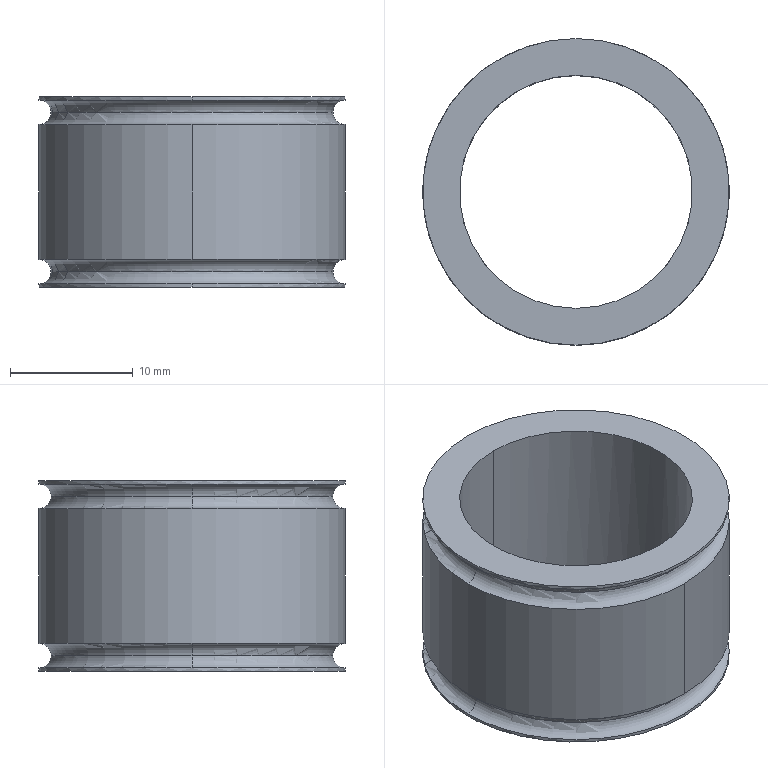Part | NX | 1 solid | 20 faces | box 25 x 25 x 15.5 mm | volume 2973 mm3 | cylinder 8 | torus 8 | plane 2 | cone 2 | commonest cylinder face diameters 25 x6 19 x2
STEP:
#1=CARTESIAN_POINT('',(-140.,184.2,-49.75));
#2=VERTEX_POINT('',#1);
#3=CARTESIAN_POINT('',(-140.,209.2,-49.75));
#4=VERTEX_POINT('',#3);
#5=CARTESIAN_POINT('',(-140.,196.7,-49.75));
#6=DIRECTION('',(0.,0.,1.));
#7=DIRECTION('',(0.,-1.,0.));
#8=AXIS2_PLACEMENT_3D('',#5,#6,#7);
#9=CIRCLE('',#8,12.5);
#10=EDGE_CURVE('',#2,#4,#9,.T.);
#11=ORIENTED_EDGE('',*,*,#10,.F.);
#12=CARTESIAN_POINT('',(-140.,196.7,-49.75));
#13=DIRECTION('',(0.,0.,1.));
#14=DIRECTION('',(0.,-1.,0.));
#15=AXIS2_PLACEMENT_3D('',#12,#13,#14);
#16=CIRCLE('',#15,12.5);
#17=EDGE_CURVE('',#4,#2,#16,.T.);
#18=ORIENTED_EDGE('',*,*,#17,.F.);
#19=EDGE_LOOP('',(#11,#18));
#20=FACE_BOUND('',#19,.T.);
#21=CARTESIAN_POINT('',(-130.2,196.7,-49.75));
#22=VERTEX_POINT('',#21);
#23=CARTESIAN_POINT('',(-149.8,196.7,-49.75));
#24=VERTEX_POINT('',#23);
#25=CARTESIAN_POINT('',(-140.,196.7,-49.75));
#26=DIRECTION('',(0.,0.,1.));
#27=DIRECTION('',(0.,-1.,0.));
#28=AXIS2_PLACEMENT_3D('',#25,#26,#27);
#29=CIRCLE('',#28,9.8);
#30=EDGE_CURVE('',#22,#24,#29,.T.);
#31=ORIENTED_EDGE('',*,*,#30,.T.);
#32=CARTESIAN_POINT('',(-140.,196.7,-49.75));
#33=DIRECTION('',(0.,0.,1.));
#34=DIRECTION('',(0.,-1.,0.));
#35=AXIS2_PLACEMENT_3D('',#32,#33,#34);
#36=CIRCLE('',#35,9.8);
#37=EDGE_CURVE('',#24,#22,#36,.T.);
#38=ORIENTED_EDGE('',*,*,#37,.T.);
#39=EDGE_LOOP('',(#31,#38));
#40=FACE_BOUND('',#39,.T.);
#41=CARTESIAN_POINT('',(-140.,205.45,-49.75));
#42=DIRECTION('',(0.,0.,-1.));
#43=DIRECTION('',(-1.,0.,0.));
#44=AXIS2_PLACEMENT_3D('',#41,#42,#43);
#45=PLANE('',#44);
#46=ADVANCED_FACE('',(#20,#40),#45,.T.);
#47=CARTESIAN_POINT('',(-140.,206.2,-34.25));
#48=VERTEX_POINT('',#47);
#49=CARTESIAN_POINT('',(-140.,187.2,-34.25));
#50=VERTEX_POINT('',#49);
#51=CARTESIAN_POINT('',(-140.,196.7,-34.25));
#52=DIRECTION('',(0.,0.,1.));
#53=DIRECTION('',(0.,-1.,0.));
#54=AXIS2_PLACEMENT_3D('',#51,#52,#53);
#55=CIRCLE('',#54,9.5);
#56=EDGE_CURVE('',#48,#50,#55,.T.);
#57=ORIENTED_EDGE('',*,*,#56,.T.);
#58=CARTESIAN_POINT('',(-140.,187.2,-49.45));
#59=VERTEX_POINT('',#58);
#60=CARTESIAN_POINT('',(-140.,187.2,-42.));
#61=DIRECTION('',(0.,0.,1.));
#62=VECTOR('',#61,1000.);
#63=LINE('',#60,#62);
#64=EDGE_CURVE('',#50,#59,#63,.F.);
#65=ORIENTED_EDGE('',*,*,#64,.T.);
#66=CARTESIAN_POINT('',(-149.5,196.7,-49.45));
#67=VERTEX_POINT('',#66);
#68=CARTESIAN_POINT('',(-140.,196.7,-49.45));
#69=DIRECTION('',(0.,0.,1.));
#70=DIRECTION('',(0.,-1.,0.));
#71=AXIS2_PLACEMENT_3D('',#68,#69,#70);
#72=CIRCLE('',#71,9.5);
#73=EDGE_CURVE('',#67,#59,#72,.T.);
#74=ORIENTED_EDGE('',*,*,#73,.F.);
#75=CARTESIAN_POINT('',(-140.,206.2,-49.45));
#76=VERTEX_POINT('',#75);
#77=CARTESIAN_POINT('',(-140.,196.7,-49.45));
#78=DIRECTION('',(0.,0.,1.));
#79=DIRECTION('',(0.,-1.,0.));
#80=AXIS2_PLACEMENT_3D('',#77,#78,#79);
#81=CIRCLE('',#80,9.5);
#82=EDGE_CURVE('',#76,#67,#81,.T.);
#83=ORIENTED_EDGE('',*,*,#82,.F.);
#84=CARTESIAN_POINT('',(-140.,206.2,-42.));
#85=DIRECTION('',(0.,0.,1.));
#86=VECTOR('',#85,1000.);
#87=LINE('',#84,#86);
#88=EDGE_CURVE('',#48,#76,#87,.F.);
#89=ORIENTED_EDGE('',*,*,#88,.F.);
#90=EDGE_LOOP('',(#57,#65,#74,#83,#89));
#91=FACE_BOUND('',#90,.T.);
#92=CARTESIAN_POINT('',(-140.,196.7,-42.));
#93=DIRECTION('',(0.,0.,1.));
#94=DIRECTION('',(0.,-1.,0.));
#95=AXIS2_PLACEMENT_3D('',#92,#93,#94);
#96=CYLINDRICAL_SURFACE('',#95,9.5);
#97=ADVANCED_FACE('',(#91),#96,.F.);
#98=CARTESIAN_POINT('',(-140.,209.2,-34.25));
#99=VERTEX_POINT('',#98);
#100=CARTESIAN_POINT('',(-140.,184.2,-34.25));
#101=VERTEX_POINT('',#100);
#102=CARTESIAN_POINT('',(-140.,196.7,-34.25));
#103=DIRECTION('',(0.,0.,1.));
#104=DIRECTION('',(0.,-1.,0.));
#105=AXIS2_PLACEMENT_3D('',#102,#103,#104);
#106=CIRCLE('',#105,12.5);
#107=EDGE_CURVE('',#99,#101,#106,.T.);
#108=ORIENTED_EDGE('',*,*,#107,.T.);
#109=CARTESIAN_POINT('',(-140.,196.7,-34.25));
#110=DIRECTION('',(0.,0.,1.));
#111=DIRECTION('',(0.,-1.,0.));
#112=AXIS2_PLACEMENT_3D('',#109,#110,#111);
#113=CIRCLE('',#112,12.5);
#114=EDGE_CURVE('',#101,#99,#113,.T.);
#115=ORIENTED_EDGE('',*,*,#114,.T.);
#116=EDGE_LOOP('',(#108,#115));
#117=FACE_BOUND('',#116,.T.);
#118=ORIENTED_EDGE('',*,*,#56,.F.);
#119=CARTESIAN_POINT('',(-140.,196.7,-34.25));
#120=DIRECTION('',(0.,0.,1.));
#121=DIRECTION('',(0.,-1.,0.));
#122=AXIS2_PLACEMENT_3D('',#119,#120,#121);
#123=CIRCLE('',#122,9.5);
#124=EDGE_CURVE('',#50,#48,#123,.T.);
#125=ORIENTED_EDGE('',*,*,#124,.F.);
#126=EDGE_LOOP('',(#118,#125));
#127=FACE_BOUND('',#126,.T.);
#128=CARTESIAN_POINT('',(-140.,205.45,-34.25));
#129=DIRECTION('',(0.,0.,1.));
#130=DIRECTION('',(1.,0.,0.));
#131=AXIS2_PLACEMENT_3D('',#128,#129,#130);
#132=PLANE('',#131);
#133=ADVANCED_FACE('',(#117,#127),#132,.T.);
#134=CARTESIAN_POINT('',(-127.5,196.7,-49.5));
#135=VERTEX_POINT('',#134);
#136=CARTESIAN_POINT('',(-140.,209.2,-49.5));
#137=VERTEX_POINT('',#136);
#138=CARTESIAN_POINT('',(-140.,196.7,-49.5));
#139=DIRECTION('',(0.,0.,1.));
#140=DIRECTION('',(1.,0.,0.));
#141=AXIS2_PLACEMENT_3D('',#138,#139,#140);
#142=CIRCLE('',#141,12.5);
#143=EDGE_CURVE('',#135,#137,#142,.T.);
#144=ORIENTED_EDGE('',*,*,#143,.F.);
#145=CARTESIAN_POINT('',(-140.,184.2,-49.5));
#146=VERTEX_POINT('',#145);
#147=CARTESIAN_POINT('',(-140.,196.7,-49.5));
#148=DIRECTION('',(0.,0.,1.));
#149=DIRECTION('',(1.,0.,0.));
#150=AXIS2_PLACEMENT_3D('',#147,#148,#149);
#151=CIRCLE('',#150,12.5);
#152=EDGE_CURVE('',#146,#135,#151,.T.);
#153=ORIENTED_EDGE('',*,*,#152,.F.);
#154=CARTESIAN_POINT('',(-140.,184.2,-42.));
#155=DIRECTION('',(0.,0.,1.));
#156=VECTOR('',#155,1000.);
#157=LINE('',#154,#156);
#158=EDGE_CURVE('',#2,#146,#157,.T.);
#159=ORIENTED_EDGE('',*,*,#158,.F.);
#160=ORIENTED_EDGE('',*,*,#10,.T.);
#161=CARTESIAN_POINT('',(-140.,209.2,-42.));
#162=DIRECTION('',(0.,0.,1.));
#163=VECTOR('',#162,1000.);
#164=LINE('',#161,#163);
#165=EDGE_CURVE('',#4,#137,#164,.T.);
#166=ORIENTED_EDGE('',*,*,#165,.T.);
#167=EDGE_LOOP('',(#144,#153,#159,#160,#166));
#168=FACE_BOUND('',#167,.T.);
#169=CARTESIAN_POINT('',(-140.,196.7,-42.));
#170=DIRECTION('',(0.,0.,1.));
#171=DIRECTION('',(0.,-1.,0.));
#172=AXIS2_PLACEMENT_3D('',#169,#170,#171);
#173=CYLINDRICAL_SURFACE('',#172,12.5);
#174=ADVANCED_FACE('',(#168),#173,.T.);
#175=CARTESIAN_POINT('',(-127.5,196.7,-34.5));
#176=VERTEX_POINT('',#175);
#177=CARTESIAN_POINT('',(-140.,209.2,-34.5));
#178=VERTEX_POINT('',#177);
#179=CARTESIAN_POINT('',(-140.,196.7,-34.5));
#180=DIRECTION('',(0.,0.,1.));
#181=DIRECTION('',(1.,0.,0.));
#182=AXIS2_PLACEMENT_3D('',#179,#180,#181);
#183=CIRCLE('',#182,12.5);
#184=EDGE_CURVE('',#176,#178,#183,.T.);
#185=ORIENTED_EDGE('',*,*,#184,.T.);
#186=CARTESIAN_POINT('',(-140.,209.2,-42.));
#187=DIRECTION('',(0.,0.,1.));
#188=VECTOR('',#187,1000.);
#189=LINE('',#186,#188);
#190=EDGE_CURVE('',#178,#99,#189,.T.);
#191=ORIENTED_EDGE('',*,*,#190,.T.);
#192=ORIENTED_EDGE('',*,*,#114,.F.);
#193=CARTESIAN_POINT('',(-140.,184.2,-34.5));
#194=VERTEX_POINT('',#193);
#195=CARTESIAN_POINT('',(-140.,184.2,-42.));
#196=DIRECTION('',(0.,0.,1.));
#197=VECTOR('',#196,1000.);
#198=LINE('',#195,#197);
#199=EDGE_CURVE('',#194,#101,#198,.T.);
#200=ORIENTED_EDGE('',*,*,#199,.F.);
#201=CARTESIAN_POINT('',(-140.,196.7,-34.5));
#202=DIRECTION('',(0.,0.,1.));
#203=DIRECTION('',(1.,0.,0.));
#204=AXIS2_PLACEMENT_3D('',#201,#202,#203);
#205=CIRCLE('',#204,12.5);
#206=EDGE_CURVE('',#194,#176,#205,.T.);
#207=ORIENTED_EDGE('',*,*,#206,.T.);
#208=EDGE_LOOP('',(#185,#191,#192,#200,#207));
#209=FACE_BOUND('',#208,.T.);
#210=CARTESIAN_POINT('',(-140.,196.7,-42.));
#211=DIRECTION('',(0.,0.,1.));
#212=DIRECTION('',(0.,-1.,0.));
#213=AXIS2_PLACEMENT_3D('',#210,#211,#212);
#214=CYLINDRICAL_SURFACE('',#213,12.5);
#215=ADVANCED_FACE('',(#209),#214,.T.);
#216=CARTESIAN_POINT('',(-127.5,196.7,-47.5));
#217=VERTEX_POINT('',#216);
#218=CARTESIAN_POINT('',(-140.,209.2,-47.5));
#219=VERTEX_POINT('',#218);
#220=CARTESIAN_POINT('',(-140.,196.7,-47.5));
#221=DIRECTION('',(0.,0.,1.));
#222=DIRECTION('',(1.,0.,0.));
#223=AXIS2_PLACEMENT_3D('',#220,#221,#222);
#224=CIRCLE('',#223,12.5);
#225=EDGE_CURVE('',#217,#219,#224,.T.);
#226=ORIENTED_EDGE('',*,*,#225,.T.);
#227=CARTESIAN_POINT('',(-140.,209.2,-36.5));
#228=VERTEX_POINT('',#227);
#229=CARTESIAN_POINT('',(-140.,209.2,-42.));
#230=DIRECTION('',(0.,0.,1.));
#231=VECTOR('',#230,1000.);
#232=LINE('',#229,#231);
#233=EDGE_CURVE('',#219,#228,#232,.T.);
#234=ORIENTED_EDGE('',*,*,#233,.T.);
#235=CARTESIAN_POINT('',(-127.5,196.7,-36.5));
#236=VERTEX_POINT('',#235);
#237=CARTESIAN_POINT('',(-140.,196.7,-36.5));
#238=DIRECTION('',(0.,0.,1.));
#239=DIRECTION('',(1.,0.,0.));
#240=AXIS2_PLACEMENT_3D('',#237,#238,#239);
#241=CIRCLE('',#240,12.5);
#242=EDGE_CURVE('',#236,#228,#241,.T.);
#243=ORIENTED_EDGE('',*,*,#242,.F.);
#244=CARTESIAN_POINT('',(-140.,184.2,-36.5));
#245=VERTEX_POINT('',#244);
#246=CARTESIAN_POINT('',(-140.,196.7,-36.5));
#247=DIRECTION('',(0.,0.,1.));
#248=DIRECTION('',(1.,0.,0.));
#249=AXIS2_PLACEMENT_3D('',#246,#247,#248);
#250=CIRCLE('',#249,12.5);
#251=EDGE_CURVE('',#245,#236,#250,.T.);
#252=ORIENTED_EDGE('',*,*,#251,.F.);
#253=CARTESIAN_POINT('',(-140.,184.2,-47.5));
#254=VERTEX_POINT('',#253);
#255=CARTESIAN_POINT('',(-140.,184.2,-42.));
#256=DIRECTION('',(0.,0.,1.));
#257=VECTOR('',#256,1000.);
#258=LINE('',#255,#257);
#259=EDGE_CURVE('',#254,#245,#258,.T.);
#260=ORIENTED_EDGE('',*,*,#259,.F.);
#261=CARTESIAN_POINT('',(-140.,196.7,-47.5));
#262=DIRECTION('',(0.,0.,1.));
#263=DIRECTION('',(1.,0.,0.));
#264=AXIS2_PLACEMENT_3D('',#261,#262,#263);
#265=CIRCLE('',#264,12.5);
#266=EDGE_CURVE('',#254,#217,#265,.T.);
#267=ORIENTED_EDGE('',*,*,#266,.T.);
#268=EDGE_LOOP('',(#226,#234,#243,#252,#260,#267));
#269=FACE_BOUND('',#268,.T.);
#270=CARTESIAN_POINT('',(-140.,196.7,-42.));
#271=DIRECTION('',(0.,0.,1.));
#272=DIRECTION('',(0.,-1.,0.));
#273=AXIS2_PLACEMENT_3D('',#270,#271,#272);
#274=CYLINDRICAL_SURFACE('',#273,12.5);
#275=ADVANCED_FACE('',(#269),#274,.T.);
#276=CARTESIAN_POINT('',(-128.5,196.7,-48.5));
#277=VERTEX_POINT('',#276);
#278=CARTESIAN_POINT('',(-151.5,196.7,-48.5));
#279=VERTEX_POINT('',#278);
#280=CARTESIAN_POINT('',(-140.,196.7,-48.5));
#281=DIRECTION('',(0.,0.,1.));
#282=DIRECTION('',(0.,-1.,0.));
#283=AXIS2_PLACEMENT_3D('',#280,#281,#282);
#284=CIRCLE('',#283,11.5);
#285=EDGE_CURVE('',#277,#279,#284,.T.);
#286=ORIENTED_EDGE('',*,*,#285,.F.);
#287=CARTESIAN_POINT('',(-127.5,196.7,-48.5));
#288=DIRECTION('',(0.,1.,0.));
#289=DIRECTION('',(0.,0.,-1.));
#290=AXIS2_PLACEMENT_3D('',#287,#288,#289);
#291=CIRCLE('',#290,1.);
#292=EDGE_CURVE('',#277,#135,#291,.F.);
#293=ORIENTED_EDGE('',*,*,#292,.T.);
#294=ORIENTED_EDGE('',*,*,#143,.T.);
#295=CARTESIAN_POINT('',(-152.5,196.7,-49.5));
#296=VERTEX_POINT('',#295);
#297=CARTESIAN_POINT('',(-140.,196.7,-49.5));
#298=DIRECTION('',(0.,0.,1.));
#299=DIRECTION('',(1.,0.,0.));
#300=AXIS2_PLACEMENT_3D('',#297,#298,#299);
#301=CIRCLE('',#300,12.5);
#302=EDGE_CURVE('',#137,#296,#301,.T.);
#303=ORIENTED_EDGE('',*,*,#302,.T.);
#304=CARTESIAN_POINT('',(-152.5,196.7,-48.5));
#305=DIRECTION('',(0.,-1.,0.));
#306=DIRECTION('',(0.,0.,-1.));
#307=AXIS2_PLACEMENT_3D('',#304,#305,#306);
#308=CIRCLE('',#307,1.);
#309=EDGE_CURVE('',#279,#296,#308,.F.);
#310=ORIENTED_EDGE('',*,*,#309,.F.);
#311=EDGE_LOOP('',(#286,#293,#294,#303,#310));
#312=FACE_BOUND('',#311,.T.);
#313=CARTESIAN_POINT('',(-140.,196.7,-48.5));
#314=DIRECTION('',(0.,0.,1.));
#315=DIRECTION('',(1.,0.,0.));
#316=AXIS2_PLACEMENT_3D('',#313,#314,#315);
#317=TOROIDAL_SURFACE('',#316,12.5,1.);
#318=ADVANCED_FACE('',(#312),#317,.F.);
#319=CARTESIAN_POINT('',(-128.5,196.7,-35.5));
#320=VERTEX_POINT('',#319);
#321=CARTESIAN_POINT('',(-151.5,196.7,-35.5));
#322=VERTEX_POINT('',#321);
#323=CARTESIAN_POINT('',(-140.,196.7,-35.5));
#324=DIRECTION('',(0.,0.,1.));
#325=DIRECTION('',(0.,-1.,0.));
#326=AXIS2_PLACEMENT_3D('',#323,#324,#325);
#327=CIRCLE('',#326,11.5);
#328=EDGE_CURVE('',#320,#322,#327,.T.);
#329=ORIENTED_EDGE('',*,*,#328,.F.);
#330=CARTESIAN_POINT('',(-127.5,196.7,-35.5));
#331=DIRECTION('',(0.,1.,0.));
#332=DIRECTION('',(0.,0.,-1.));
#333=AXIS2_PLACEMENT_3D('',#330,#331,#332);
#334=CIRCLE('',#333,1.);
#335=EDGE_CURVE('',#320,#236,#334,.F.);
#336=ORIENTED_EDGE('',*,*,#335,.T.);
#337=ORIENTED_EDGE('',*,*,#242,.T.);
#338=CARTESIAN_POINT('',(-152.5,196.7,-36.5));
#339=VERTEX_POINT('',#338);
#340=CARTESIAN_POINT('',(-140.,196.7,-36.5));
#341=DIRECTION('',(0.,0.,1.));
#342=DIRECTION('',(1.,0.,0.));
#343=AXIS2_PLACEMENT_3D('',#340,#341,#342);
#344=CIRCLE('',#343,12.5);
#345=EDGE_CURVE('',#228,#339,#344,.T.);
#346=ORIENTED_EDGE('',*,*,#345,.T.);
#347=CARTESIAN_POINT('',(-152.5,196.7,-35.5));
#348=DIRECTION('',(0.,-1.,0.));
#349=DIRECTION('',(0.,0.,-1.));
#350=AXIS2_PLACEMENT_3D('',#347,#348,#349);
#351=CIRCLE('',#350,1.);
#352=EDGE_CURVE('',#322,#339,#351,.F.);
#353=ORIENTED_EDGE('',*,*,#352,.F.);
#354=EDGE_LOOP('',(#329,#336,#337,#346,#353));
#355=FACE_BOUND('',#354,.T.);
#356=CARTESIAN_POINT('',(-140.,196.7,-35.5));
#357=DIRECTION('',(0.,0.,1.));
#358=DIRECTION('',(1.,0.,0.));
#359=AXIS2_PLACEMENT_3D('',#356,#357,#358);
#360=TOROIDAL_SURFACE('',#359,12.5,1.);
#361=ADVANCED_FACE('',(#355),#360,.F.);
#362=ORIENTED_EDGE('',*,*,#30,.F.);
#363=CARTESIAN_POINT('',(-130.5,196.7,-49.45));
#364=VERTEX_POINT('',#363);
#365=CARTESIAN_POINT('',(-130.2,196.7,-49.75));
#366=DIRECTION('',(0.7071,0.,-0.7071));
#367=VECTOR('',#366,1000.);
#368=LINE('',#365,#367);
#369=EDGE_CURVE('',#22,#364,#368,.F.);
#370=ORIENTED_EDGE('',*,*,#369,.T.);
#371=CARTESIAN_POINT('',(-140.,196.7,-49.45));
#372=DIRECTION('',(0.,0.,1.));
#373=DIRECTION('',(0.,-1.,0.));
#374=AXIS2_PLACEMENT_3D('',#371,#372,#373);
#375=CIRCLE('',#374,9.5);
#376=EDGE_CURVE('',#364,#76,#375,.T.);
#377=ORIENTED_EDGE('',*,*,#376,.T.);
#378=ORIENTED_EDGE('',*,*,#82,.T.);
#379=CARTESIAN_POINT('',(-149.8,196.7,-49.75));
#380=DIRECTION('',(-0.7071,0.,-0.7071));
#381=VECTOR('',#380,1000.);
#382=LINE('',#379,#381);
#383=EDGE_CURVE('',#24,#67,#382,.F.);
#384=ORIENTED_EDGE('',*,*,#383,.F.);
#385=EDGE_LOOP('',(#362,#370,#377,#378,#384));
#386=FACE_BOUND('',#385,.T.);
#387=CARTESIAN_POINT('',(-140.,196.7,-49.75));
#388=DIRECTION('',(0.,0.,-1.));
#389=DIRECTION('',(-1.,0.,0.));
#390=AXIS2_PLACEMENT_3D('',#387,#388,#389);
#391=CONICAL_SURFACE('',#390,9.8,0.7854);
#392=ADVANCED_FACE('',(#386),#391,.F.);
#393=CARTESIAN_POINT('',(-140.,196.7,-36.5));
#394=DIRECTION('',(0.,0.,1.));
#395=DIRECTION('',(1.,0.,0.));
#396=AXIS2_PLACEMENT_3D('',#393,#394,#395);
#397=CIRCLE('',#396,12.5);
#398=EDGE_CURVE('',#339,#245,#397,.T.);
#399=ORIENTED_EDGE('',*,*,#398,.F.);
#400=ORIENTED_EDGE('',*,*,#345,.F.);
#401=ORIENTED_EDGE('',*,*,#233,.F.);
#402=CARTESIAN_POINT('',(-152.5,196.7,-47.5));
#403=VERTEX_POINT('',#402);
#404=CARTESIAN_POINT('',(-140.,196.7,-47.5));
#405=DIRECTION('',(0.,0.,1.));
#406=DIRECTION('',(1.,0.,0.));
#407=AXIS2_PLACEMENT_3D('',#404,#405,#406);
#408=CIRCLE('',#407,12.5);
#409=EDGE_CURVE('',#219,#403,#408,.T.);
#410=ORIENTED_EDGE('',*,*,#409,.T.);
#411=CARTESIAN_POINT('',(-140.,196.7,-47.5));
#412=DIRECTION('',(0.,0.,1.));
#413=DIRECTION('',(1.,0.,0.));
#414=AXIS2_PLACEMENT_3D('',#411,#412,#413);
#415=CIRCLE('',#414,12.5);
#416=EDGE_CURVE('',#403,#254,#415,.T.);
#417=ORIENTED_EDGE('',*,*,#416,.T.);
#418=ORIENTED_EDGE('',*,*,#259,.T.);
#419=EDGE_LOOP('',(#399,#400,#401,#410,#417,#418));
#420=FACE_BOUND('',#419,.T.);
#421=CARTESIAN_POINT('',(-140.,196.7,-42.));
#422=DIRECTION('',(0.,0.,1.));
#423=DIRECTION('',(0.,-1.,0.));
#424=AXIS2_PLACEMENT_3D('',#421,#422,#423);
#425=CYLINDRICAL_SURFACE('',#424,12.5);
#426=ADVANCED_FACE('',(#420),#425,.T.);
#427=ORIENTED_EDGE('',*,*,#107,.F.);
#428=ORIENTED_EDGE('',*,*,#190,.F.);
#429=CARTESIAN_POINT('',(-152.5,196.7,-34.5));
#430=VERTEX_POINT('',#429);
#431=CARTESIAN_POINT('',(-140.,196.7,-34.5));
#432=DIRECTION('',(0.,0.,1.));
#433=DIRECTION('',(1.,0.,0.));
#434=AXIS2_PLACEMENT_3D('',#431,#432,#433);
#435=CIRCLE('',#434,12.5);
#436=EDGE_CURVE('',#178,#430,#435,.T.);
#437=ORIENTED_EDGE('',*,*,#436,.T.);
#438=CARTESIAN_POINT('',(-140.,196.7,-34.5));
#439=DIRECTION('',(0.,0.,1.));
#440=DIRECTION('',(1.,0.,0.));
#441=AXIS2_PLACEMENT_3D('',#438,#439,#440);
#442=CIRCLE('',#441,12.5);
#443=EDGE_CURVE('',#430,#194,#442,.T.);
#444=ORIENTED_EDGE('',*,*,#443,.T.);
#445=ORIENTED_EDGE('',*,*,#199,.T.);
#446=EDGE_LOOP('',(#427,#428,#437,#444,#445));
#447=FACE_BOUND('',#446,.T.);
#448=CARTESIAN_POINT('',(-140.,196.7,-42.));
#449=DIRECTION('',(0.,0.,1.));
#450=DIRECTION('',(0.,-1.,0.));
#451=AXIS2_PLACEMENT_3D('',#448,#449,#450);
#452=CYLINDRICAL_SURFACE('',#451,12.5);
#453=ADVANCED_FACE('',(#447),#452,.T.);
#454=ORIENTED_EDGE('',*,*,#376,.F.);
#455=CARTESIAN_POINT('',(-140.,196.7,-49.45));
#456=DIRECTION('',(0.,0.,1.));
#457=DIRECTION('',(0.,-1.,0.));
#458=AXIS2_PLACEMENT_3D('',#455,#456,#457);
#459=CIRCLE('',#458,9.5);
#460=EDGE_CURVE('',#59,#364,#459,.T.);
#461=ORIENTED_EDGE('',*,*,#460,.F.);
#462=ORIENTED_EDGE('',*,*,#64,.F.);
#463=ORIENTED_EDGE('',*,*,#124,.T.);
#464=ORIENTED_EDGE('',*,*,#88,.T.);
#465=EDGE_LOOP('',(#454,#461,#462,#463,#464));
#466=FACE_BOUND('',#465,.T.);
#467=CARTESIAN_POINT('',(-140.,196.7,-42.));
#468=DIRECTION('',(0.,0.,1.));
#469=DIRECTION('',(0.,-1.,0.));
#470=AXIS2_PLACEMENT_3D('',#467,#468,#469);
#471=CYLINDRICAL_SURFACE('',#470,9.5);
#472=ADVANCED_FACE('',(#466),#471,.F.);
#473=ORIENTED_EDGE('',*,*,#383,.T.);
#474=ORIENTED_EDGE('',*,*,#73,.T.);
#475=ORIENTED_EDGE('',*,*,#460,.T.);
#476=ORIENTED_EDGE('',*,*,#369,.F.);
#477=ORIENTED_EDGE('',*,*,#37,.F.);
#478=EDGE_LOOP('',(#473,#474,#475,#476,#477));
#479=FACE_BOUND('',#478,.T.);
#480=CARTESIAN_POINT('',(-140.,196.7,-49.75));
#481=DIRECTION('',(0.,0.,-1.));
#482=DIRECTION('',(-1.,0.,0.));
#483=AXIS2_PLACEMENT_3D('',#480,#481,#482);
#484=CONICAL_SURFACE('',#483,9.8,0.7854);
#485=ADVANCED_FACE('',(#479),#484,.F.);
#486=ORIENTED_EDGE('',*,*,#165,.F.);
#487=ORIENTED_EDGE('',*,*,#17,.T.);
#488=ORIENTED_EDGE('',*,*,#158,.T.);
#489=CARTESIAN_POINT('',(-140.,196.7,-49.5));
#490=DIRECTION('',(0.,0.,1.));
#491=DIRECTION('',(1.,0.,0.));
#492=AXIS2_PLACEMENT_3D('',#489,#490,#491);
#493=CIRCLE('',#492,12.5);
#494=EDGE_CURVE('',#296,#146,#493,.T.);
#495=ORIENTED_EDGE('',*,*,#494,.F.);
#496=ORIENTED_EDGE('',*,*,#302,.F.);
#497=EDGE_LOOP('',(#486,#487,#488,#495,#496));
#498=FACE_BOUND('',#497,.T.);
#499=CARTESIAN_POINT('',(-140.,196.7,-42.));
#500=DIRECTION('',(0.,0.,1.));
#501=DIRECTION('',(0.,-1.,0.));
#502=AXIS2_PLACEMENT_3D('',#499,#500,#501);
#503=CYLINDRICAL_SURFACE('',#502,12.5);
#504=ADVANCED_FACE('',(#498),#503,.T.);
#505=CARTESIAN_POINT('',(-140.,196.7,-35.5));
#506=DIRECTION('',(0.,0.,1.));
#507=DIRECTION('',(0.,-1.,0.));
#508=AXIS2_PLACEMENT_3D('',#505,#506,#507);
#509=CIRCLE('',#508,11.5);
#510=EDGE_CURVE('',#322,#320,#509,.T.);
#511=ORIENTED_EDGE('',*,*,#510,.F.);
#512=ORIENTED_EDGE('',*,*,#352,.T.);
#513=ORIENTED_EDGE('',*,*,#398,.T.);
#514=ORIENTED_EDGE('',*,*,#251,.T.);
#515=ORIENTED_EDGE('',*,*,#335,.F.);
#516=EDGE_LOOP('',(#511,#512,#513,#514,#515));
#517=FACE_BOUND('',#516,.T.);
#518=CARTESIAN_POINT('',(-140.,196.7,-35.5));
#519=DIRECTION('',(0.,0.,1.));
#520=DIRECTION('',(1.,0.,0.));
#521=AXIS2_PLACEMENT_3D('',#518,#519,#520);
#522=TOROIDAL_SURFACE('',#521,12.5,1.);
#523=ADVANCED_FACE('',(#517),#522,.F.);
#524=CARTESIAN_POINT('',(-140.,196.7,-48.5));
#525=DIRECTION('',(0.,0.,1.));
#526=DIRECTION('',(0.,-1.,0.));
#527=AXIS2_PLACEMENT_3D('',#524,#525,#526);
#528=CIRCLE('',#527,11.5);
#529=EDGE_CURVE('',#279,#277,#528,.T.);
#530=ORIENTED_EDGE('',*,*,#529,.F.);
#531=ORIENTED_EDGE('',*,*,#309,.T.);
#532=ORIENTED_EDGE('',*,*,#494,.T.);
#533=ORIENTED_EDGE('',*,*,#152,.T.);
#534=ORIENTED_EDGE('',*,*,#292,.F.);
#535=EDGE_LOOP('',(#530,#531,#532,#533,#534));
#536=FACE_BOUND('',#535,.T.);
#537=CARTESIAN_POINT('',(-140.,196.7,-48.5));
#538=DIRECTION('',(0.,0.,1.));
#539=DIRECTION('',(1.,0.,0.));
#540=AXIS2_PLACEMENT_3D('',#537,#538,#539);
#541=TOROIDAL_SURFACE('',#540,12.5,1.);
#542=ADVANCED_FACE('',(#536),#541,.F.);
#543=CARTESIAN_POINT('',(-152.5,196.7,-48.5));
#544=DIRECTION('',(0.,-1.,0.));
#545=DIRECTION('',(0.,0.,-1.));
#546=AXIS2_PLACEMENT_3D('',#543,#544,#545);
#547=CIRCLE('',#546,1.);
#548=EDGE_CURVE('',#279,#403,#547,.T.);
#549=ORIENTED_EDGE('',*,*,#548,.F.);
#550=ORIENTED_EDGE('',*,*,#529,.T.);
#551=CARTESIAN_POINT('',(-127.5,196.7,-48.5));
#552=DIRECTION('',(0.,1.,0.));
#553=DIRECTION('',(0.,0.,-1.));
#554=AXIS2_PLACEMENT_3D('',#551,#552,#553);
#555=CIRCLE('',#554,1.);
#556=EDGE_CURVE('',#277,#217,#555,.T.);
#557=ORIENTED_EDGE('',*,*,#556,.T.);
#558=ORIENTED_EDGE('',*,*,#266,.F.);
#559=ORIENTED_EDGE('',*,*,#416,.F.);
#560=EDGE_LOOP('',(#549,#550,#557,#558,#559));
#561=FACE_BOUND('',#560,.T.);
#562=CARTESIAN_POINT('',(-140.,196.7,-48.5));
#563=DIRECTION('',(0.,0.,1.));
#564=DIRECTION('',(1.,0.,0.));
#565=AXIS2_PLACEMENT_3D('',#562,#563,#564);
#566=TOROIDAL_SURFACE('',#565,12.5,1.);
#567=ADVANCED_FACE('',(#561),#566,.F.);
#568=CARTESIAN_POINT('',(-152.5,196.7,-35.5));
#569=DIRECTION('',(0.,-1.,0.));
#570=DIRECTION('',(0.,0.,-1.));
#571=AXIS2_PLACEMENT_3D('',#568,#569,#570);
#572=CIRCLE('',#571,1.);
#573=EDGE_CURVE('',#322,#430,#572,.T.);
#574=ORIENTED_EDGE('',*,*,#573,.F.);
#575=ORIENTED_EDGE('',*,*,#510,.T.);
#576=CARTESIAN_POINT('',(-127.5,196.7,-35.5));
#577=DIRECTION('',(0.,1.,0.));
#578=DIRECTION('',(0.,0.,-1.));
#579=AXIS2_PLACEMENT_3D('',#576,#577,#578);
#580=CIRCLE('',#579,1.);
#581=EDGE_CURVE('',#320,#176,#580,.T.);
#582=ORIENTED_EDGE('',*,*,#581,.T.);
#583=ORIENTED_EDGE('',*,*,#206,.F.);
#584=ORIENTED_EDGE('',*,*,#443,.F.);
#585=EDGE_LOOP('',(#574,#575,#582,#583,#584));
#586=FACE_BOUND('',#585,.T.);
#587=CARTESIAN_POINT('',(-140.,196.7,-35.5));
#588=DIRECTION('',(0.,0.,1.));
#589=DIRECTION('',(1.,0.,0.));
#590=AXIS2_PLACEMENT_3D('',#587,#588,#589);
#591=TOROIDAL_SURFACE('',#590,12.5,1.);
#592=ADVANCED_FACE('',(#586),#591,.F.);
#593=ORIENTED_EDGE('',*,*,#581,.F.);
#594=ORIENTED_EDGE('',*,*,#328,.T.);
#595=ORIENTED_EDGE('',*,*,#573,.T.);
#596=ORIENTED_EDGE('',*,*,#436,.F.);
#597=ORIENTED_EDGE('',*,*,#184,.F.);
#598=EDGE_LOOP('',(#593,#594,#595,#596,#597));
#599=FACE_BOUND('',#598,.T.);
#600=CARTESIAN_POINT('',(-140.,196.7,-35.5));
#601=DIRECTION('',(0.,0.,1.));
#602=DIRECTION('',(1.,0.,0.));
#603=AXIS2_PLACEMENT_3D('',#600,#601,#602);
#604=TOROIDAL_SURFACE('',#603,12.5,1.);
#605=ADVANCED_FACE('',(#599),#604,.F.);
#606=ORIENTED_EDGE('',*,*,#556,.F.);
#607=ORIENTED_EDGE('',*,*,#285,.T.);
#608=ORIENTED_EDGE('',*,*,#548,.T.);
#609=ORIENTED_EDGE('',*,*,#409,.F.);
#610=ORIENTED_EDGE('',*,*,#225,.F.);
#611=EDGE_LOOP('',(#606,#607,#608,#609,#610));
#612=FACE_BOUND('',#611,.T.);
#613=CARTESIAN_POINT('',(-140.,196.7,-48.5));
#614=DIRECTION('',(0.,0.,1.));
#615=DIRECTION('',(1.,0.,0.));
#616=AXIS2_PLACEMENT_3D('',#613,#614,#615);
#617=TOROIDAL_SURFACE('',#616,12.5,1.);
#618=ADVANCED_FACE('',(#612),#617,.F.);
#619=CLOSED_SHELL('',(#46,#97,#133,#174,#215,#275,#318,#361,#392,#426,#453,#472,#485,#504,#523,#542,#567,#592,#605,#618));
#620=MANIFOLD_SOLID_BREP('',#619);
#621=(LENGTH_UNIT()NAMED_UNIT(*)SI_UNIT(.MILLI.,.METRE.));
#622=UNCERTAINTY_MEASURE_WITH_UNIT(LENGTH_MEASURE(0.00001),#621,'','');
#623=(NAMED_UNIT(*)PLANE_ANGLE_UNIT()SI_UNIT($,.RADIAN.));
#624=(NAMED_UNIT(*)SI_UNIT($,.STERADIAN.)SOLID_ANGLE_UNIT());
#625=(GEOMETRIC_REPRESENTATION_CONTEXT(3)GLOBAL_UNCERTAINTY_ASSIGNED_CONTEXT((#622))GLOBAL_UNIT_ASSIGNED_CONTEXT((#621,#623,#624))REPRESENTATION_CONTEXT('',''));
#626=ADVANCED_BREP_SHAPE_REPRESENTATION('',(#620),#625);